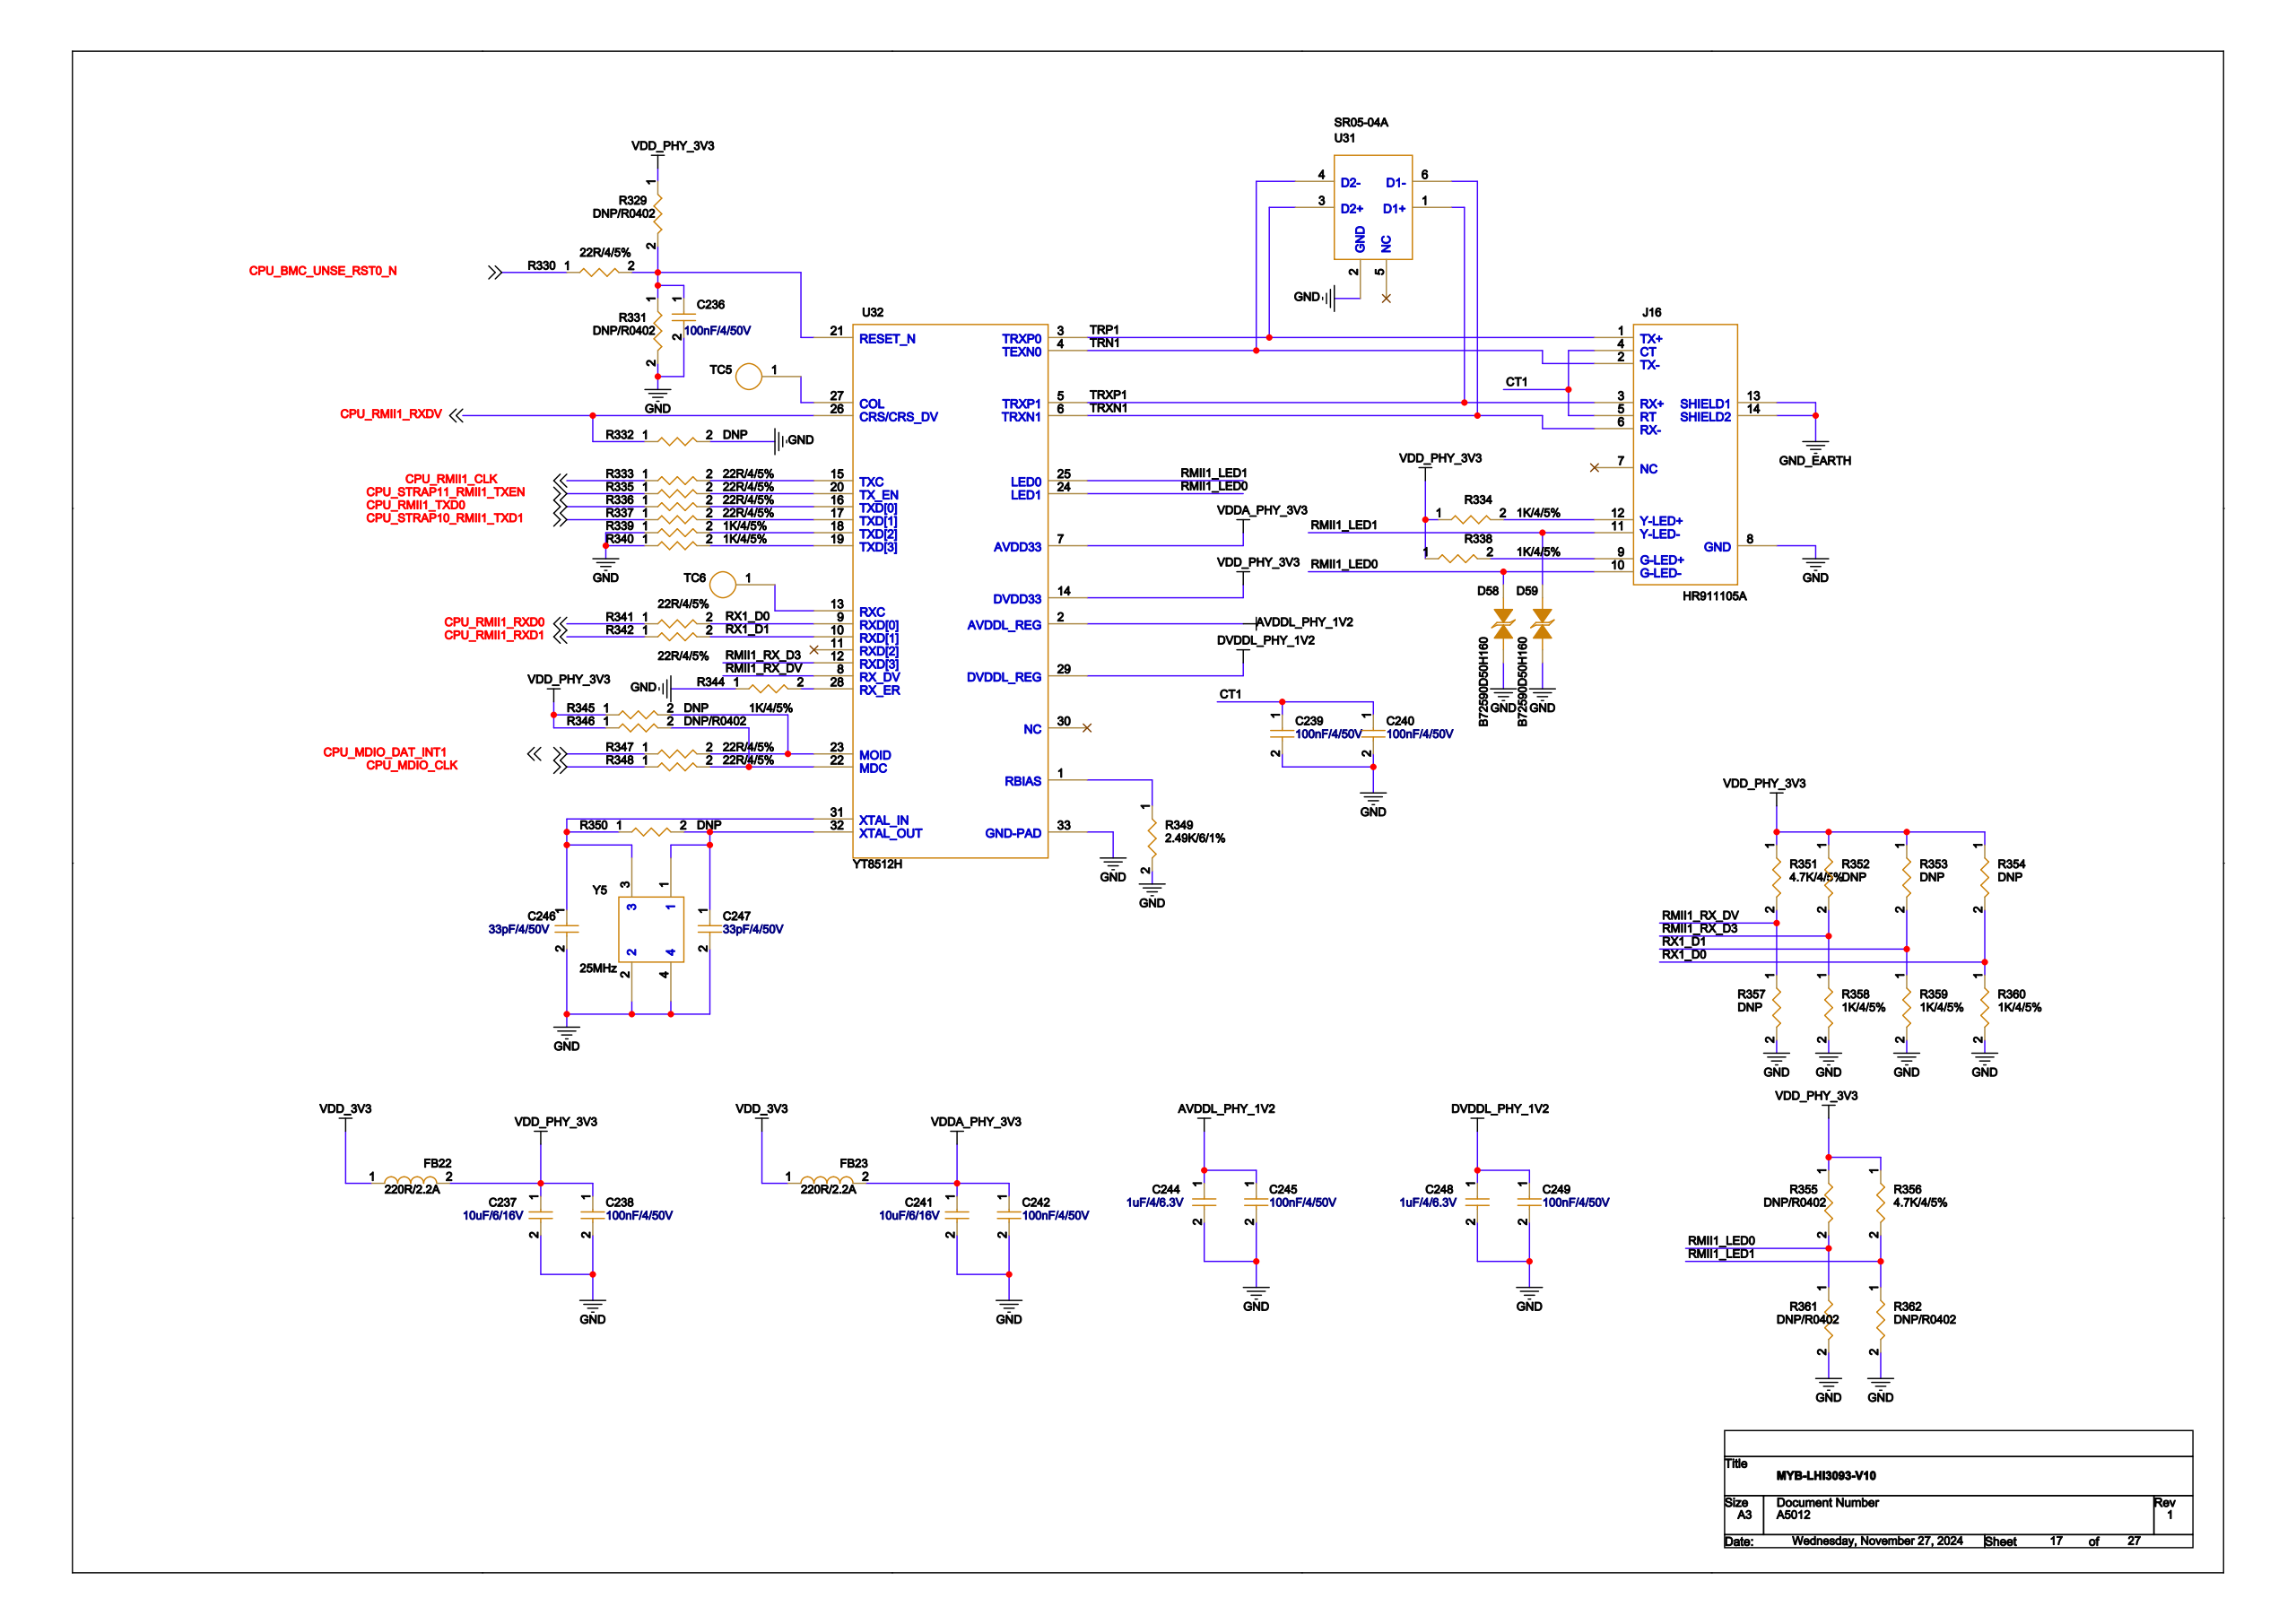Circuit board | Cadence Allegro | 1159 parts | 708 nets | one sheet of the schematic
Parts on this sheet (reference | value | footprint):
C236 | 100nF/4/50V | C0402
C237 | 10uF/6/16V | C0603
C238 | 100nF/4/50V | C0402
C239 | 100nF/4/50V | C0402
C240 | 100nF/4/50V | C0402
C241 | 10uF/6/16V | C0603
C242 | 100nF/4/50V | C0402
C244 | 1uF/4/6.3V | C0402
C245 | 100nF/4/50V | C0402
C246 | 33pF/4/50V | C0402
C247 | 33pF/4/50V | C0402
C248 | 1uF/4/6.3V | C0402
C249 | 100nF/4/50V | C0402
D59 | B72590D50H160 | D0402
FB22 | 220R/2.2A | FB0603
FB23 | 220R/2.2A | FB0603
J16 | HR911105A | RJ45-HR91105A
R329 | DNP/R0402 | R0402
R330 | 22R/4/5% | R0402
R331 | DNP/R0402 | R0402
R332 | DNP | R0402
R333 | 22R/4/5% | R0402
R334 | 1K/4/5% | R0402
R335 | 22R/4/5% | R0402
R336 | 22R/4/5% | R0402
R337 | 22R/4/5% | R0402
R338 | 1K/4/5% | R0402
R339 | 1K/4/5% | R0402
R340 | 1K/4/5% | R0402
R341 | 22R/4/5% | R0402
R342 | 22R/4/5% | R0402
R344 | 1K/4/5% | R0402
R345 | DNP | R0402
R346 | DNP/R0402 | R0402
R347 | 22R/4/5% | R0402
R348 | 22R/4/5% | R0402
R349 | 2.49K/6/1% | R0402
R350 | DNP | R0402
R351 | 4.7K/4/5% | R0402
R352 | DNP | R0402
R353 | DNP | R0402
R354 | DNP | R0402
R355 | DNP/R0402 | R0402
R356 | 4.7K/4/5% | R0402
R357 | DNP | R0402
R358 | 1K/4/5% | R0402
R359 | 1K/4/5% | R0402
R360 | 1K/4/5% | R0402
R361 | DNP/R0402 | R0402
R362 | DNP/R0402 | R0402
TC5 | TP | TP_SMT
TC6 | TP | TP_SMT
U32 | YT8512H | QFN32
Y5 | 25MHz | 3225
Nets of these parts (net: part-pin ...):
GND: C236-2 C237-2 C238-2 C239-2 C240-2 C241-2 C242-2 C244-2 C245-2 C246-2 C247-2 C248-2 C249-2 D59-1 J16-8 R331-2 R332-2 R339-1 R340-1 R344-1 R349-2 R357-2 R358-2 R359-2 R360-2 R361-2 R362-2 Y5-2 Y5-4 U32-33
VDD_3V3: FB22-1 FB23-1
N15028813: C236-1 R329-2 R330-2 R331-1 U32-21
VDD_PHY_3V3: C237-1 C238-1 FB22-2 R329-1 R334-1 R338-1 R345-1 R346-1 R351-1 R352-1 R353-1 R354-1 R355-1 R356-1 U32-14
CT1: C239-1 C240-1 J16-4 J16-5
VDDA_PHY_3V3: C241-1 C242-1 FB23-2 U32-7
AVDDL_PHY_1V2: C244-1 C245-1 U32-2
DVDDL_PHY_1V2: C248-1 C249-1 U32-29
GND_EARTH: J16-13 J16-14
N15028101: C246-1 R350-1 Y5-3 U32-31
N15028013: C247-1 R350-2 Y5-1 U32-32
RMII1_LED0: J16-10 R355-2 R361-1 U32-24
RMII1_LED1: D59-2 J16-11 R356-2 R362-1 U32-25
N15026597: J16-12 R334-2
N15026727: J16-9 R338-2
N15028689: R339-2 U32-18
N15028693: R340-2 U32-19
N15027841: R344-2 U32-28
RMII1_RX_D3: R352-2 R358-1 U32-12
RX1_D1: R342-2 R353-2 R359-1 U32-10
RX1_D0: R341-2 R354-2 R360-1 U32-9
CPU_STRAP10_RMII1_TXD1: R337-1
CPU_MDIO_CLK: R348-1
CPU_MDIO_DAT_INT1: R347-1
CPU_BMC_UNSE_RST0_N: R330-1
CPU_RMII1_CLK: R333-1
N15028649: R333-2 U32-15
CPU_STRAP11_RMII1_TXEN: R335-1
N15028653: R335-2 U32-20
CPU_RMII1_TXD0: R336-1
N15028681: R336-2 U32-16
N15028685: R337-2 U32-17
CPU_RMII1_RXD0: R341-1
CPU_RMII1_RXD1: R342-1
N15027893: R345-2 R347-2 U32-23
N15027897: R346-2 R348-2 U32-22
RMII1_RX_DV: R351-2 R357-1 U32-8
CPU_RMII1_RXDV: R332-1 U32-26
N15028197: R349-1 U32-1
N15028777: TC5-1 U32-27
N15028769: TC6-1 U32-13
TRXP1: J16-3 U32-5
TRXN1: J16-6 U32-6
TRP1: J16-1 U32-3
TRN1: J16-2 U32-4